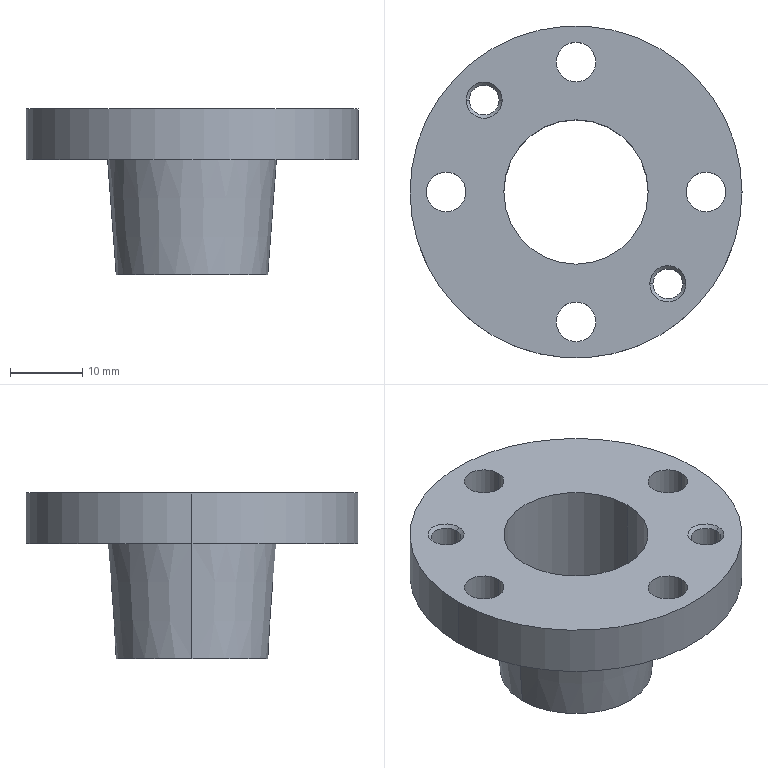Part | STEP file | LFSP35B_20_boltbushing | 1 solid | 29 faces | box 46 x 46 x 23 mm | volume 9749 mm3 | cylinder 16 | cone 10 | plane 3 | commonest cylinder face diameters 5.5 x8 4.134 x4 20 x2 46 x2